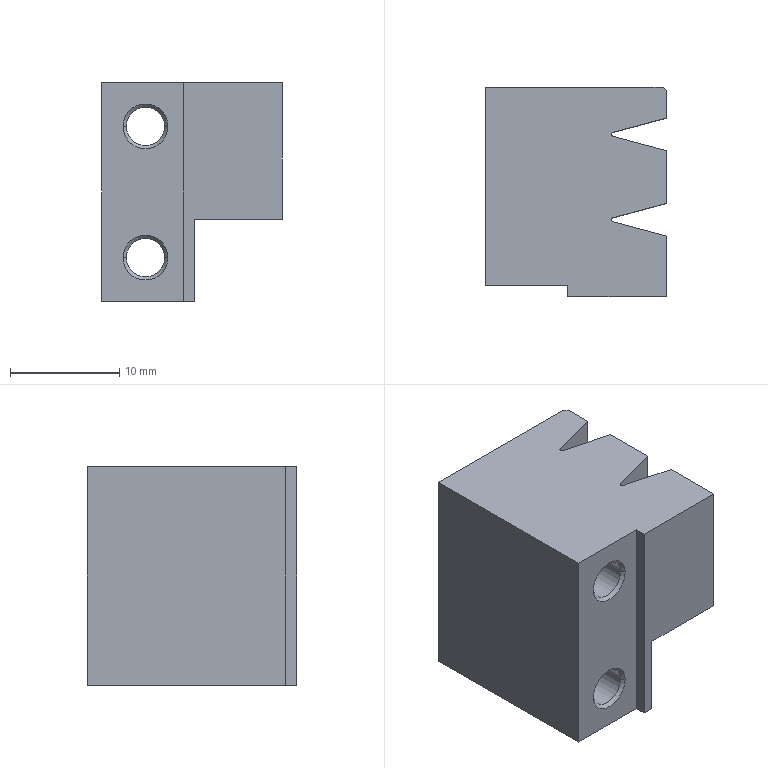Part | NX | 1 solid | 37 faces | box 16.5 x 19.1 x 20 mm | volume 4184 mm3 | plane 19 | cylinder 10 | cone 8 | commonest cylinder face diameters 3.5 x4 6 x4 0.4 x2
STEP:
#1=CARTESIAN_POINT('',(0.,9.05,-2.5));
#2=VERTEX_POINT('',#1);
#3=CARTESIAN_POINT('',(0.,-10.05,-2.5));
#4=VERTEX_POINT('',#3);
#5=CARTESIAN_POINT('',(0.,0.,-2.5));
#6=DIRECTION('',(0.,-1.,0.));
#7=VECTOR('',#6,1000.);
#8=LINE('',#5,#7);
#9=EDGE_CURVE('',#2,#4,#8,.T.);
#10=ORIENTED_EDGE('',*,*,#9,.F.);
#11=CARTESIAN_POINT('',(7.7,9.05,-2.5));
#12=VERTEX_POINT('',#11);
#13=CARTESIAN_POINT('',(0.,9.05,-2.5));
#14=DIRECTION('',(1.,0.,0.));
#15=VECTOR('',#14,1000.);
#16=LINE('',#13,#15);
#17=EDGE_CURVE('',#2,#12,#16,.T.);
#18=ORIENTED_EDGE('',*,*,#17,.T.);
#19=CARTESIAN_POINT('',(8.,8.75,-2.5));
#20=VERTEX_POINT('',#19);
#21=CARTESIAN_POINT('',(16.75,0.,-2.5));
#22=DIRECTION('',(-0.7071,0.7071,0.));
#23=VECTOR('',#22,1000.);
#24=LINE('',#21,#23);
#25=EDGE_CURVE('',#20,#12,#24,.T.);
#26=ORIENTED_EDGE('',*,*,#25,.F.);
#27=CARTESIAN_POINT('',(8.,6.247,-2.5));
#28=VERTEX_POINT('',#27);
#29=CARTESIAN_POINT('',(8.,0.,-2.5));
#30=DIRECTION('',(0.,1.,0.));
#31=VECTOR('',#30,1000.);
#32=LINE('',#29,#31);
#33=EDGE_CURVE('',#28,#20,#32,.T.);
#34=ORIENTED_EDGE('',*,*,#33,.F.);
#35=CARTESIAN_POINT('',(3.132,4.943,-2.5));
#36=VERTEX_POINT('',#35);
#37=CARTESIAN_POINT('',(0.,4.104,-2.5));
#38=DIRECTION('',(-0.9659,-0.2588,0.));
#39=VECTOR('',#38,1000.);
#40=LINE('',#37,#39);
#41=EDGE_CURVE('',#28,#36,#40,.T.);
#42=ORIENTED_EDGE('',*,*,#41,.T.);
#43=CARTESIAN_POINT('',(3.132,4.557,-2.5));
#44=VERTEX_POINT('',#43);
#45=CARTESIAN_POINT('',(3.184,4.75,-2.5));
#46=DIRECTION('',(0.,0.,-1.));
#47=DIRECTION('',(0.,1.,0.));
#48=AXIS2_PLACEMENT_3D('',#45,#46,#47);
#49=CIRCLE('',#48,0.2);
#50=EDGE_CURVE('',#44,#36,#49,.T.);
#51=ORIENTED_EDGE('',*,*,#50,.F.);
#52=CARTESIAN_POINT('',(8.,3.253,-2.5));
#53=VERTEX_POINT('',#52);
#54=CARTESIAN_POINT('',(0.,5.396,-2.5));
#55=DIRECTION('',(0.9659,-0.2588,0.));
#56=VECTOR('',#55,1000.);
#57=LINE('',#54,#56);
#58=EDGE_CURVE('',#44,#53,#57,.T.);
#59=ORIENTED_EDGE('',*,*,#58,.T.);
#60=CARTESIAN_POINT('',(8.,-1.553,-2.5));
#61=VERTEX_POINT('',#60);
#62=CARTESIAN_POINT('',(8.,0.,-2.5));
#63=DIRECTION('',(0.,1.,0.));
#64=VECTOR('',#63,1000.);
#65=LINE('',#62,#64);
#66=EDGE_CURVE('',#61,#53,#65,.T.);
#67=ORIENTED_EDGE('',*,*,#66,.F.);
#68=CARTESIAN_POINT('',(3.132,-2.857,-2.5));
#69=VERTEX_POINT('',#68);
#70=CARTESIAN_POINT('',(0.,-3.696,-2.5));
#71=DIRECTION('',(-0.9659,-0.2588,0.));
#72=VECTOR('',#71,1000.);
#73=LINE('',#70,#72);
#74=EDGE_CURVE('',#61,#69,#73,.T.);
#75=ORIENTED_EDGE('',*,*,#74,.T.);
#76=CARTESIAN_POINT('',(3.132,-3.243,-2.5));
#77=VERTEX_POINT('',#76);
#78=CARTESIAN_POINT('',(3.184,-3.05,-2.5));
#79=DIRECTION('',(0.,0.,-1.));
#80=DIRECTION('',(0.,1.,0.));
#81=AXIS2_PLACEMENT_3D('',#78,#79,#80);
#82=CIRCLE('',#81,0.2);
#83=EDGE_CURVE('',#77,#69,#82,.T.);
#84=ORIENTED_EDGE('',*,*,#83,.F.);
#85=CARTESIAN_POINT('',(8.,-4.547,-2.5));
#86=VERTEX_POINT('',#85);
#87=CARTESIAN_POINT('',(0.,-2.404,-2.5));
#88=DIRECTION('',(0.9659,-0.2588,0.));
#89=VECTOR('',#88,1000.);
#90=LINE('',#87,#89);
#91=EDGE_CURVE('',#77,#86,#90,.T.);
#92=ORIENTED_EDGE('',*,*,#91,.T.);
#93=CARTESIAN_POINT('',(8.,-10.05,-2.5));
#94=VERTEX_POINT('',#93);
#95=CARTESIAN_POINT('',(8.,0.,-2.5));
#96=DIRECTION('',(0.,1.,0.));
#97=VECTOR('',#96,1000.);
#98=LINE('',#95,#97);
#99=EDGE_CURVE('',#94,#86,#98,.T.);
#100=ORIENTED_EDGE('',*,*,#99,.F.);
#101=CARTESIAN_POINT('',(0.,-10.05,-2.5));
#102=DIRECTION('',(-1.,0.,0.));
#103=VECTOR('',#102,1000.);
#104=LINE('',#101,#103);
#105=EDGE_CURVE('',#94,#4,#104,.T.);
#106=ORIENTED_EDGE('',*,*,#105,.T.);
#107=EDGE_LOOP('',(#10,#18,#26,#34,#42,#51,#59,#67,#75,#84,#92,#100,#106));
#108=FACE_BOUND('',#107,.T.);
#109=CARTESIAN_POINT('',(8.7,-11.96,-2.5));
#110=DIRECTION('',(0.,0.,1.));
#111=DIRECTION('',(1.,0.,0.));
#112=AXIS2_PLACEMENT_3D('',#109,#110,#111);
#113=PLANE('',#112);
#114=ADVANCED_FACE('',(#108),#113,.F.);
#115=CARTESIAN_POINT('',(0.,-10.05,-10.));
#116=VERTEX_POINT('',#115);
#117=CARTESIAN_POINT('',(-1.,-10.05,-10.));
#118=VERTEX_POINT('',#117);
#119=CARTESIAN_POINT('',(0.,-10.05,-10.));
#120=DIRECTION('',(-1.,0.,0.));
#121=VECTOR('',#120,1000.);
#122=LINE('',#119,#121);
#123=EDGE_CURVE('',#116,#118,#122,.T.);
#124=ORIENTED_EDGE('',*,*,#123,.F.);
#125=CARTESIAN_POINT('',(0.,-10.05,0.));
#126=DIRECTION('',(0.,0.,-1.));
#127=VECTOR('',#126,1000.);
#128=LINE('',#125,#127);
#129=EDGE_CURVE('',#4,#116,#128,.T.);
#130=ORIENTED_EDGE('',*,*,#129,.F.);
#131=ORIENTED_EDGE('',*,*,#105,.F.);
#132=CARTESIAN_POINT('',(8.,-10.05,10.));
#133=VERTEX_POINT('',#132);
#134=CARTESIAN_POINT('',(8.,-10.05,0.));
#135=DIRECTION('',(0.,0.,1.));
#136=VECTOR('',#135,1000.);
#137=LINE('',#134,#136);
#138=EDGE_CURVE('',#94,#133,#137,.T.);
#139=ORIENTED_EDGE('',*,*,#138,.T.);
#140=CARTESIAN_POINT('',(-1.,-10.05,10.));
#141=VERTEX_POINT('',#140);
#142=CARTESIAN_POINT('',(0.,-10.05,10.));
#143=DIRECTION('',(-1.,0.,0.));
#144=VECTOR('',#143,1000.);
#145=LINE('',#142,#144);
#146=EDGE_CURVE('',#133,#141,#145,.T.);
#147=ORIENTED_EDGE('',*,*,#146,.T.);
#148=CARTESIAN_POINT('',(-1.,-10.05,0.));
#149=DIRECTION('',(0.,0.,1.));
#150=VECTOR('',#149,1000.);
#151=LINE('',#148,#150);
#152=EDGE_CURVE('',#118,#141,#151,.T.);
#153=ORIENTED_EDGE('',*,*,#152,.F.);
#154=EDGE_LOOP('',(#124,#130,#131,#139,#147,#153));
#155=FACE_BOUND('',#154,.T.);
#156=CARTESIAN_POINT('',(1.648,-10.05,2.608));
#157=DIRECTION('',(0.,-1.,0.));
#158=DIRECTION('',(0.,0.,-1.));
#159=AXIS2_PLACEMENT_3D('',#156,#157,#158);
#160=PLANE('',#159);
#161=ADVANCED_FACE('',(#155),#160,.T.);
#162=ORIENTED_EDGE('',*,*,#9,.T.);
#163=ORIENTED_EDGE('',*,*,#129,.T.);
#164=CARTESIAN_POINT('',(0.,9.05,-10.));
#165=VERTEX_POINT('',#164);
#166=CARTESIAN_POINT('',(0.,0.,-10.));
#167=DIRECTION('',(0.,-1.,0.));
#168=VECTOR('',#167,1000.);
#169=LINE('',#166,#168);
#170=EDGE_CURVE('',#165,#116,#169,.T.);
#171=ORIENTED_EDGE('',*,*,#170,.F.);
#172=CARTESIAN_POINT('',(0.,9.05,0.));
#173=DIRECTION('',(0.,0.,-1.));
#174=VECTOR('',#173,1000.);
#175=LINE('',#172,#174);
#176=EDGE_CURVE('',#2,#165,#175,.T.);
#177=ORIENTED_EDGE('',*,*,#176,.F.);
#178=EDGE_LOOP('',(#162,#163,#171,#177));
#179=FACE_BOUND('',#178,.T.);
#180=CARTESIAN_POINT('',(0.,-9.05,0.));
#181=DIRECTION('',(1.,0.,0.));
#182=DIRECTION('',(0.,1.,0.));
#183=AXIS2_PLACEMENT_3D('',#180,#181,#182);
#184=PLANE('',#183);
#185=ADVANCED_FACE('',(#179),#184,.T.);
#186=ORIENTED_EDGE('',*,*,#66,.T.);
#187=CARTESIAN_POINT('',(8.,3.253,10.));
#188=VERTEX_POINT('',#187);
#189=CARTESIAN_POINT('',(8.,3.253,0.));
#190=DIRECTION('',(0.,0.,-1.));
#191=VECTOR('',#190,1000.);
#192=LINE('',#189,#191);
#193=EDGE_CURVE('',#188,#53,#192,.T.);
#194=ORIENTED_EDGE('',*,*,#193,.F.);
#195=CARTESIAN_POINT('',(8.,-1.553,10.));
#196=VERTEX_POINT('',#195);
#197=CARTESIAN_POINT('',(8.,0.,10.));
#198=DIRECTION('',(0.,1.,0.));
#199=VECTOR('',#198,1000.);
#200=LINE('',#197,#199);
#201=EDGE_CURVE('',#196,#188,#200,.T.);
#202=ORIENTED_EDGE('',*,*,#201,.F.);
#203=CARTESIAN_POINT('',(8.,-1.553,0.));
#204=DIRECTION('',(0.,0.,-1.));
#205=VECTOR('',#204,1000.);
#206=LINE('',#203,#205);
#207=EDGE_CURVE('',#196,#61,#206,.T.);
#208=ORIENTED_EDGE('',*,*,#207,.T.);
#209=EDGE_LOOP('',(#186,#194,#202,#208));
#210=FACE_BOUND('',#209,.T.);
#211=CARTESIAN_POINT('',(8.,5.432,0.));
#212=DIRECTION('',(1.,0.,0.));
#213=DIRECTION('',(0.,1.,0.));
#214=AXIS2_PLACEMENT_3D('',#211,#212,#213);
#215=PLANE('',#214);
#216=ADVANCED_FACE('',(#210),#215,.T.);
#217=CARTESIAN_POINT('',(-1.,-9.05,10.));
#218=VERTEX_POINT('',#217);
#219=CARTESIAN_POINT('',(-1.,0.,10.));
#220=DIRECTION('',(0.,1.,0.));
#221=VECTOR('',#220,1000.);
#222=LINE('',#219,#221);
#223=EDGE_CURVE('',#141,#218,#222,.T.);
#224=ORIENTED_EDGE('',*,*,#223,.F.);
#225=ORIENTED_EDGE('',*,*,#146,.F.);
#226=CARTESIAN_POINT('',(8.,-4.547,10.));
#227=VERTEX_POINT('',#226);
#228=CARTESIAN_POINT('',(8.,0.,10.));
#229=DIRECTION('',(0.,-1.,0.));
#230=VECTOR('',#229,1000.);
#231=LINE('',#228,#230);
#232=EDGE_CURVE('',#227,#133,#231,.T.);
#233=ORIENTED_EDGE('',*,*,#232,.F.);
#234=CARTESIAN_POINT('',(3.132,-3.243,10.));
#235=VERTEX_POINT('',#234);
#236=CARTESIAN_POINT('',(0.,-2.404,10.));
#237=DIRECTION('',(-0.9659,0.2588,0.));
#238=VECTOR('',#237,1000.);
#239=LINE('',#236,#238);
#240=EDGE_CURVE('',#227,#235,#239,.T.);
#241=ORIENTED_EDGE('',*,*,#240,.T.);
#242=CARTESIAN_POINT('',(3.132,-2.857,10.));
#243=VERTEX_POINT('',#242);
#244=CARTESIAN_POINT('',(3.184,-3.05,10.));
#245=DIRECTION('',(0.,0.,-1.));
#246=DIRECTION('',(0.,1.,0.));
#247=AXIS2_PLACEMENT_3D('',#244,#245,#246);
#248=CIRCLE('',#247,0.2);
#249=EDGE_CURVE('',#235,#243,#248,.T.);
#250=ORIENTED_EDGE('',*,*,#249,.T.);
#251=CARTESIAN_POINT('',(0.,-3.696,10.));
#252=DIRECTION('',(0.9659,0.2588,0.));
#253=VECTOR('',#252,1000.);
#254=LINE('',#251,#253);
#255=EDGE_CURVE('',#243,#196,#254,.T.);
#256=ORIENTED_EDGE('',*,*,#255,.T.);
#257=ORIENTED_EDGE('',*,*,#201,.T.);
#258=CARTESIAN_POINT('',(3.132,4.557,10.));
#259=VERTEX_POINT('',#258);
#260=CARTESIAN_POINT('',(0.,5.396,10.));
#261=DIRECTION('',(0.9659,-0.2588,0.));
#262=VECTOR('',#261,1000.);
#263=LINE('',#260,#262);
#264=EDGE_CURVE('',#259,#188,#263,.T.);
#265=ORIENTED_EDGE('',*,*,#264,.F.);
#266=CARTESIAN_POINT('',(3.132,4.943,10.));
#267=VERTEX_POINT('',#266);
#268=CARTESIAN_POINT('',(3.184,4.75,10.));
#269=DIRECTION('',(0.,0.,-1.));
#270=DIRECTION('',(0.,1.,0.));
#271=AXIS2_PLACEMENT_3D('',#268,#269,#270);
#272=CIRCLE('',#271,0.2);
#273=EDGE_CURVE('',#259,#267,#272,.T.);
#274=ORIENTED_EDGE('',*,*,#273,.T.);
#275=CARTESIAN_POINT('',(8.,6.247,10.));
#276=VERTEX_POINT('',#275);
#277=CARTESIAN_POINT('',(0.,4.104,10.));
#278=DIRECTION('',(0.9659,0.2588,0.));
#279=VECTOR('',#278,1000.);
#280=LINE('',#277,#279);
#281=EDGE_CURVE('',#267,#276,#280,.T.);
#282=ORIENTED_EDGE('',*,*,#281,.T.);
#283=CARTESIAN_POINT('',(8.,8.75,10.));
#284=VERTEX_POINT('',#283);
#285=CARTESIAN_POINT('',(8.,0.,10.));
#286=DIRECTION('',(0.,1.,0.));
#287=VECTOR('',#286,1000.);
#288=LINE('',#285,#287);
#289=EDGE_CURVE('',#276,#284,#288,.T.);
#290=ORIENTED_EDGE('',*,*,#289,.T.);
#291=CARTESIAN_POINT('',(7.7,9.05,10.));
#292=VERTEX_POINT('',#291);
#293=CARTESIAN_POINT('',(16.75,0.,10.));
#294=DIRECTION('',(-0.7071,0.7071,0.));
#295=VECTOR('',#294,1000.);
#296=LINE('',#293,#295);
#297=EDGE_CURVE('',#284,#292,#296,.T.);
#298=ORIENTED_EDGE('',*,*,#297,.T.);
#299=CARTESIAN_POINT('',(-8.5,9.05,10.));
#300=VERTEX_POINT('',#299);
#301=CARTESIAN_POINT('',(0.,9.05,10.));
#302=DIRECTION('',(1.,0.,0.));
#303=VECTOR('',#302,1000.);
#304=LINE('',#301,#303);
#305=EDGE_CURVE('',#300,#292,#304,.T.);
#306=ORIENTED_EDGE('',*,*,#305,.F.);
#307=CARTESIAN_POINT('',(-8.5,-9.05,10.));
#308=VERTEX_POINT('',#307);
#309=CARTESIAN_POINT('',(-8.5,0.,10.));
#310=DIRECTION('',(0.,1.,0.));
#311=VECTOR('',#310,1000.);
#312=LINE('',#309,#311);
#313=EDGE_CURVE('',#308,#300,#312,.T.);
#314=ORIENTED_EDGE('',*,*,#313,.F.);
#315=CARTESIAN_POINT('',(0.,-9.05,10.));
#316=DIRECTION('',(-1.,0.,0.));
#317=VECTOR('',#316,1000.);
#318=LINE('',#315,#317);
#319=EDGE_CURVE('',#218,#308,#318,.T.);
#320=ORIENTED_EDGE('',*,*,#319,.F.);
#321=EDGE_LOOP('',(#224,#225,#233,#241,#250,#256,#257,#265,#274,#282,#290,#298,#306,#314,#320));
#322=FACE_BOUND('',#321,.T.);
#323=CARTESIAN_POINT('',(-1.,-9.05,10.));
#324=DIRECTION('',(0.,0.,1.));
#325=DIRECTION('',(1.,0.,0.));
#326=AXIS2_PLACEMENT_3D('',#323,#324,#325);
#327=PLANE('',#326);
#328=ADVANCED_FACE('',(#322),#327,.T.);
#329=CARTESIAN_POINT('',(-6.55,-9.05,-6.));
#330=VERTEX_POINT('',#329);
#331=CARTESIAN_POINT('',(-2.45,-9.05,-6.));
#332=VERTEX_POINT('',#331);
#333=CARTESIAN_POINT('',(-4.5,-9.05,-6.));
#334=DIRECTION('',(0.,-1.,0.));
#335=DIRECTION('',(-1.,0.,0.));
#336=AXIS2_PLACEMENT_3D('',#333,#334,#335);
#337=CIRCLE('',#336,2.05);
#338=EDGE_CURVE('',#330,#332,#337,.T.);
#339=ORIENTED_EDGE('',*,*,#338,.T.);
#340=CARTESIAN_POINT('',(-2.75,-8.75,-6.));
#341=VERTEX_POINT('',#340);
#342=CARTESIAN_POINT('',(-2.45,-9.05,-6.));
#343=DIRECTION('',(0.7071,-0.7071,0.));
#344=VECTOR('',#343,1000.);
#345=LINE('',#342,#344);
#346=EDGE_CURVE('',#332,#341,#345,.F.);
#347=ORIENTED_EDGE('',*,*,#346,.T.);
#348=CARTESIAN_POINT('',(-6.25,-8.75,-6.));
#349=VERTEX_POINT('',#348);
#350=CARTESIAN_POINT('',(-4.5,-8.75,-6.));
#351=DIRECTION('',(0.,-1.,0.));
#352=DIRECTION('',(-1.,0.,0.));
#353=AXIS2_PLACEMENT_3D('',#350,#351,#352);
#354=CIRCLE('',#353,1.75);
#355=EDGE_CURVE('',#349,#341,#354,.T.);
#356=ORIENTED_EDGE('',*,*,#355,.F.);
#357=CARTESIAN_POINT('',(-6.55,-9.05,-6.));
#358=DIRECTION('',(-0.7071,-0.7071,0.));
#359=VECTOR('',#358,1000.);
#360=LINE('',#357,#359);
#361=EDGE_CURVE('',#330,#349,#360,.F.);
#362=ORIENTED_EDGE('',*,*,#361,.F.);
#363=EDGE_LOOP('',(#339,#347,#356,#362));
#364=FACE_BOUND('',#363,.T.);
#365=CARTESIAN_POINT('',(-4.5,-9.05,-6.));
#366=DIRECTION('',(0.,-1.,0.));
#367=DIRECTION('',(-1.,0.,0.));
#368=AXIS2_PLACEMENT_3D('',#365,#366,#367);
#369=CONICAL_SURFACE('',#368,2.05,0.7854);
#370=ADVANCED_FACE('',(#364),#369,.F.);
#371=CARTESIAN_POINT('',(7.7,9.05,0.));
#372=DIRECTION('',(0.,0.,-1.));
#373=VECTOR('',#372,1000.);
#374=LINE('',#371,#373);
#375=EDGE_CURVE('',#292,#12,#374,.T.);
#376=ORIENTED_EDGE('',*,*,#375,.T.);
#377=ORIENTED_EDGE('',*,*,#17,.F.);
#378=ORIENTED_EDGE('',*,*,#176,.T.);
#379=CARTESIAN_POINT('',(-8.5,9.05,-10.));
#380=VERTEX_POINT('',#379);
#381=CARTESIAN_POINT('',(0.,9.05,-10.));
#382=DIRECTION('',(1.,0.,0.));
#383=VECTOR('',#382,1000.);
#384=LINE('',#381,#383);
#385=EDGE_CURVE('',#380,#165,#384,.T.);
#386=ORIENTED_EDGE('',*,*,#385,.F.);
#387=CARTESIAN_POINT('',(-8.5,9.05,0.));
#388=DIRECTION('',(0.,0.,-1.));
#389=VECTOR('',#388,1000.);
#390=LINE('',#387,#389);
#391=EDGE_CURVE('',#300,#380,#390,.T.);
#392=ORIENTED_EDGE('',*,*,#391,.F.);
#393=ORIENTED_EDGE('',*,*,#305,.T.);
#394=EDGE_LOOP('',(#376,#377,#378,#386,#392,#393));
#395=FACE_BOUND('',#394,.T.);
#396=CARTESIAN_POINT('',(-1.2,9.05,6.));
#397=VERTEX_POINT('',#396);
#398=CARTESIAN_POINT('',(-7.8,9.05,6.));
#399=VERTEX_POINT('',#398);
#400=CARTESIAN_POINT('',(-4.5,9.05,6.));
#401=DIRECTION('',(0.,1.,0.));
#402=DIRECTION('',(1.,0.,0.));
#403=AXIS2_PLACEMENT_3D('',#400,#401,#402);
#404=CIRCLE('',#403,3.3);
#405=EDGE_CURVE('',#397,#399,#404,.T.);
#406=ORIENTED_EDGE('',*,*,#405,.F.);
#407=CARTESIAN_POINT('',(-4.5,9.05,6.));
#408=DIRECTION('',(0.,1.,0.));
#409=DIRECTION('',(1.,0.,0.));
#410=AXIS2_PLACEMENT_3D('',#407,#408,#409);
#411=CIRCLE('',#410,3.3);
#412=EDGE_CURVE('',#399,#397,#411,.T.);
#413=ORIENTED_EDGE('',*,*,#412,.F.);
#414=EDGE_LOOP('',(#406,#413));
#415=FACE_BOUND('',#414,.T.);
#416=CARTESIAN_POINT('',(-7.8,9.05,-6.));
#417=VERTEX_POINT('',#416);
#418=CARTESIAN_POINT('',(-1.2,9.05,-6.));
#419=VERTEX_POINT('',#418);
#420=CARTESIAN_POINT('',(-4.5,9.05,-6.));
#421=DIRECTION('',(0.,1.,0.));
#422=DIRECTION('',(1.,0.,0.));
#423=AXIS2_PLACEMENT_3D('',#420,#421,#422);
#424=CIRCLE('',#423,3.3);
#425=EDGE_CURVE('',#417,#419,#424,.T.);
#426=ORIENTED_EDGE('',*,*,#425,.F.);
#427=CARTESIAN_POINT('',(-4.5,9.05,-6.));
#428=DIRECTION('',(0.,1.,0.));
#429=DIRECTION('',(1.,0.,0.));
#430=AXIS2_PLACEMENT_3D('',#427,#428,#429);
#431=CIRCLE('',#430,3.3);
#432=EDGE_CURVE('',#419,#417,#431,.T.);
#433=ORIENTED_EDGE('',*,*,#432,.F.);
#434=EDGE_LOOP('',(#426,#433));
#435=FACE_BOUND('',#434,.T.);
#436=CARTESIAN_POINT('',(8.,9.05,-10.));
#437=DIRECTION('',(0.,1.,0.));
#438=DIRECTION('',(1.,0.,0.));
#439=AXIS2_PLACEMENT_3D('',#436,#437,#438);
#440=PLANE('',#439);
#441=ADVANCED_FACE('',(#395,#415,#435),#440,.T.);
#442=CARTESIAN_POINT('',(-4.5,1.95,-3.));
#443=VERTEX_POINT('',#442);
#444=CARTESIAN_POINT('',(-4.5,1.95,-9.));
#445=VERTEX_POINT('',#444);
#446=CARTESIAN_POINT('',(-4.5,1.95,-6.));
#447=DIRECTION('',(0.,1.,0.));
#448=DIRECTION('',(0.,0.,1.));
#449=AXIS2_PLACEMENT_3D('',#446,#447,#448);
#450=CIRCLE('',#449,3.);
#451=EDGE_CURVE('',#443,#445,#450,.T.);
#452=ORIENTED_EDGE('',*,*,#451,.T.);
#453=CARTESIAN_POINT('',(-4.5,1.95,-6.));
#454=DIRECTION('',(0.,1.,0.));
#455=DIRECTION('',(0.,0.,1.));
#456=AXIS2_PLACEMENT_3D('',#453,#454,#455);
#457=CIRCLE('',#456,3.);
#458=EDGE_CURVE('',#445,#443,#457,.T.);
#459=ORIENTED_EDGE('',*,*,#458,.T.);
#460=EDGE_LOOP('',(#452,#459));
#461=FACE_BOUND('',#460,.T.);
#462=CARTESIAN_POINT('',(-2.75,1.95,-6.));
#463=VERTEX_POINT('',#462);
#464=CARTESIAN_POINT('',(-6.25,1.95,-6.));
#465=VERTEX_POINT('',#464);
#466=CARTESIAN_POINT('',(-4.5,1.95,-6.));
#467=DIRECTION('',(0.,1.,0.));
#468=DIRECTION('',(-1.,0.,0.));
#469=AXIS2_PLACEMENT_3D('',#466,#467,#468);
#470=CIRCLE('',#469,1.75);
#471=EDGE_CURVE('',#463,#465,#470,.T.);
#472=ORIENTED_EDGE('',*,*,#471,.F.);
#473=CARTESIAN_POINT('',(-4.5,1.95,-6.));
#474=DIRECTION('',(0.,1.,0.));
#475=DIRECTION('',(-1.,0.,0.));
#476=AXIS2_PLACEMENT_3D('',#473,#474,#475);
#477=CIRCLE('',#476,1.75);
#478=EDGE_CURVE('',#465,#463,#477,.T.);
#479=ORIENTED_EDGE('',*,*,#478,.F.);
#480=EDGE_LOOP('',(#472,#479));
#481=FACE_BOUND('',#480,.T.);
#482=CARTESIAN_POINT('',(-1.269,1.95,6.939));
#483=DIRECTION('',(0.,1.,0.));
#484=DIRECTION('',(1.,0.,0.));
#485=AXIS2_PLACEMENT_3D('',#482,#483,#484);
#486=PLANE('',#485);
#487=ADVANCED_FACE('',(#461,#481),#486,.T.);
#488=CARTESIAN_POINT('',(-1.5,8.75,6.));
#489=VERTEX_POINT('',#488);
#490=CARTESIAN_POINT('',(-4.5,8.75,3.));
#491=VERTEX_POINT('',#490);
#492=CARTESIAN_POINT('',(-4.5,8.75,6.));
#493=DIRECTION('',(0.,1.,0.));
#494=DIRECTION('',(1.,0.,0.));
#495=AXIS2_PLACEMENT_3D('',#492,#493,#494);
#496=CIRCLE('',#495,3.);
#497=EDGE_CURVE('',#489,#491,#496,.T.);
#498=ORIENTED_EDGE('',*,*,#497,.F.);
#499=CARTESIAN_POINT('',(-1.5,8.75,6.));
#500=DIRECTION('',(0.7071,0.7071,0.));
#501=VECTOR('',#500,1000.);
#502=LINE('',#499,#501);
#503=EDGE_CURVE('',#397,#489,#502,.F.);
#504=ORIENTED_EDGE('',*,*,#503,.F.);
#505=ORIENTED_EDGE('',*,*,#405,.T.);
#506=CARTESIAN_POINT('',(-7.5,8.75,6.));
#507=VERTEX_POINT('',#506);
#508=CARTESIAN_POINT('',(-7.5,8.75,6.));
#509=DIRECTION('',(-0.7071,0.7071,0.));
#510=VECTOR('',#509,1000.);
#511=LINE('',#508,#510);
#512=EDGE_CURVE('',#399,#507,#511,.F.);
#513=ORIENTED_EDGE('',*,*,#512,.T.);
#514=CARTESIAN_POINT('',(-4.5,8.75,6.));
#515=DIRECTION('',(0.,1.,0.));
#516=DIRECTION('',(1.,0.,0.));
#517=AXIS2_PLACEMENT_3D('',#514,#515,#516);
#518=CIRCLE('',#517,3.);
#519=EDGE_CURVE('',#491,#507,#518,.T.);
#520=ORIENTED_EDGE('',*,*,#519,.F.);
#521=EDGE_LOOP('',(#498,#504,#505,#513,#520));
#522=FACE_BOUND('',#521,.T.);
#523=CARTESIAN_POINT('',(-4.5,8.75,6.));
#524=DIRECTION('',(0.,1.,0.));
#525=DIRECTION('',(1.,0.,0.));
#526=AXIS2_PLACEMENT_3D('',#523,#524,#525);
#527=CONICAL_SURFACE('',#526,3.,0.7854);
#528=ADVANCED_FACE('',(#522),#527,.F.);
#529=CARTESIAN_POINT('',(-6.55,-9.05,6.));
#530=VERTEX_POINT('',#529);
#531=CARTESIAN_POINT('',(-2.45,-9.05,6.));
#532=VERTEX_POINT('',#531);
#533=CARTESIAN_POINT('',(-4.5,-9.05,6.));
#534=DIRECTION('',(0.,-1.,0.));
#535=DIRECTION('',(-1.,0.,0.));
#536=AXIS2_PLACEMENT_3D('',#533,#534,#535);
#537=CIRCLE('',#536,2.05);
#538=EDGE_CURVE('',#530,#532,#537,.T.);
#539=ORIENTED_EDGE('',*,*,#538,.T.);
#540=CARTESIAN_POINT('',(-2.75,-8.75,6.));
#541=VERTEX_POINT('',#540);
#542=CARTESIAN_POINT('',(-2.45,-9.05,6.));
#543=DIRECTION('',(0.7071,-0.7071,0.));
#544=VECTOR('',#543,1000.);
#545=LINE('',#542,#544);
#546=EDGE_CURVE('',#532,#541,#545,.F.);
#547=ORIENTED_EDGE('',*,*,#546,.T.);
#548=CARTESIAN_POINT('',(-6.25,-8.75,6.));
#549=VERTEX_POINT('',#548);
#550=CARTESIAN_POINT('',(-4.5,-8.75,6.));
#551=DIRECTION('',(0.,-1.,0.));
#552=DIRECTION('',(-1.,0.,0.));
#553=AXIS2_PLACEMENT_3D('',#550,#551,#552);
#554=CIRCLE('',#553,1.75);
#555=EDGE_CURVE('',#549,#541,#554,.T.);
#556=ORIENTED_EDGE('',*,*,#555,.F.);
#557=CARTESIAN_POINT('',(-6.55,-9.05,6.));
#558=DIRECTION('',(-0.7071,-0.7071,0.));
#559=VECTOR('',#558,1000.);
#560=LINE('',#557,#559);
#561=EDGE_CURVE('',#530,#549,#560,.F.);
#562=ORIENTED_EDGE('',*,*,#561,.F.);
#563=EDGE_LOOP('',(#539,#547,#556,#562));
#564=FACE_BOUND('',#563,.T.);
#565=CARTESIAN_POINT('',(-4.5,-9.05,6.));
#566=DIRECTION('',(0.,-1.,0.));
#567=DIRECTION('',(-1.,0.,0.));
#568=AXIS2_PLACEMENT_3D('',#565,#566,#567);
#569=CONICAL_SURFACE('',#568,2.05,0.7854);
#570=ADVANCED_FACE('',(#564),#569,.F.);
#571=ORIENTED_EDGE('',*,*,#313,.T.);
#572=ORIENTED_EDGE('',*,*,#391,.T.);
#573=CARTESIAN_POINT('',(-8.5,-9.05,-10.));
#574=VERTEX_POINT('',#573);
#575=CARTESIAN_POINT('',(-8.5,0.,-10.));
#576=DIRECTION('',(0.,1.,0.));
#577=VECTOR('',#576,1000.);
#578=LINE('',#575,#577);
#579=EDGE_CURVE('',#574,#380,#578,.T.);
#580=ORIENTED_EDGE('',*,*,#579,.F.);
#581=CARTESIAN_POINT('',(-8.5,-9.05,0.));
#582=DIRECTION('',(0.,0.,1.));
#583=VECTOR('',#582,1000.);
#584=LINE('',#581,#583);
#585=EDGE_CURVE('',#574,#308,#584,.T.);
#586=ORIENTED_EDGE('',*,*,#585,.T.);
#587=EDGE_LOOP('',(#571,#572,#580,#586));
#588=FACE_BOUND('',#587,.T.);
#589=CARTESIAN_POINT('',(-8.5,9.05,-10.));
#590=DIRECTION('',(-1.,0.,0.));
#591=DIRECTION('',(0.,0.,1.));
#592=AXIS2_PLACEMENT_3D('',#589,#590,#591);
#593=PLANE('',#592);
#594=ADVANCED_FACE('',(#588),#593,.T.);
#595=CARTESIAN_POINT('',(-1.,-9.05,-10.));
#596=VERTEX_POINT('',#595);
#597=CARTESIAN_POINT('',(-1.,-9.05,0.));
#598=DIRECTION('',(0.,0.,-1.));
#599=VECTOR('',#598,1000.);
#600=LINE('',#597,#599);
#601=EDGE_CURVE('',#218,#596,#600,.T.);
#602=ORIENTED_EDGE('',*,*,#601,.F.);
#603=ORIENTED_EDGE('',*,*,#319,.T.);
#604=ORIENTED_EDGE('',*,*,#585,.F.);
#605=CARTESIAN_POINT('',(0.,-9.05,-10.));
#606=DIRECTION('',(1.,0.,0.));
#607=VECTOR('',#606,1000.);
#608=LINE('',#605,#607);
#609=EDGE_CURVE('',#574,#596,#608,.T.);
#610=ORIENTED_EDGE('',*,*,#609,.T.);
#611=EDGE_LOOP('',(#602,#603,#604,#610));
#612=FACE_BOUND('',#611,.T.);
#613=ORIENTED_EDGE('',*,*,#538,.F.);
#614=CARTESIAN_POINT('',(-4.5,-9.05,6.));
#615=DIRECTION('',(0.,-1.,0.));
#616=DIRECTION('',(-1.,0.,0.));
#617=AXIS2_PLACEMENT_3D('',#614,#615,#616);
#618=CIRCLE('',#617,2.05);
#619=EDGE_CURVE('',#532,#530,#618,.T.);
#620=ORIENTED_EDGE('',*,*,#619,.F.);
#621=EDGE_LOOP('',(#613,#620));
#622=FACE_BOUND('',#621,.T.);
#623=ORIENTED_EDGE('',*,*,#338,.F.);
#624=CARTESIAN_POINT('',(-4.5,-9.05,-6.));
#625=DIRECTION('',(0.,-1.,0.));
#626=DIRECTION('',(-1.,0.,0.));
#627=AXIS2_PLACEMENT_3D('',#624,#625,#626);
#628=CIRCLE('',#627,2.05);
#629=EDGE_CURVE('',#332,#330,#628,.T.);
#630=ORIENTED_EDGE('',*,*,#629,.F.);
#631=EDGE_LOOP('',(#623,#630));
#632=FACE_BOUND('',#631,.T.);
#633=CARTESIAN_POINT('',(-8.,-9.05,-10.));
#634=DIRECTION('',(0.,-1.,0.));
#635=DIRECTION('',(0.,0.,-1.));
#636=AXIS2_PLACEMENT_3D('',#633,#634,#635);
#637=PLANE('',#636);
#638=ADVANCED_FACE('',(#612,#622,#632),#637,.T.);
#639=ORIENTED_EDGE('',*,*,#451,.F.);
#640=CARTESIAN_POINT('',(-4.5,8.75,-3.));
#641=VERTEX_POINT('',#640);
#642=CARTESIAN_POINT('',(-4.5,9.05,-3.));
#643=DIRECTION('',(0.,1.,0.));
#644=VECTOR('',#643,1000.);
#645=LINE('',#642,#644);
#646=EDGE_CURVE('',#443,#641,#645,.T.);
#647=ORIENTED_EDGE('',*,*,#646,.T.);
#648=CARTESIAN_POINT('',(-1.5,8.75,-6.));
#649=VERTEX_POINT('',#648);
#650=CARTESIAN_POINT('',(-4.5,8.75,-6.));
#651=DIRECTION('',(0.,1.,0.));
#652=DIRECTION('',(1.,0.,0.));
#653=AXIS2_PLACEMENT_3D('',#650,#651,#652);
#654=CIRCLE('',#653,3.);
#655=EDGE_CURVE('',#641,#649,#654,.T.);
#656=ORIENTED_EDGE('',*,*,#655,.T.);
#657=CARTESIAN_POINT('',(-4.5,8.75,-9.));
#658=VERTEX_POINT('',#657);
#659=CARTESIAN_POINT('',(-4.5,8.75,-6.));
#660=DIRECTION('',(0.,1.,0.));
#661=DIRECTION('',(1.,0.,0.));
#662=AXIS2_PLACEMENT_3D('',#659,#660,#661);
#663=CIRCLE('',#662,3.);
#664=EDGE_CURVE('',#649,#658,#663,.T.);
#665=ORIENTED_EDGE('',*,*,#664,.T.);
#666=CARTESIAN_POINT('',(-4.5,9.05,-9.));
#667=DIRECTION('',(0.,1.,0.));
#668=VECTOR('',#667,1000.);
#669=LINE('',#666,#668);
#670=EDGE_CURVE('',#445,#658,#669,.T.);
#671=ORIENTED_EDGE('',*,*,#670,.F.);
#672=EDGE_LOOP('',(#639,#647,#656,#665,#671));
#673=FACE_BOUND('',#672,.T.);
#674=CARTESIAN_POINT('',(-4.5,9.05,-6.));
#675=DIRECTION('',(0.,1.,0.));
#676=DIRECTION('',(0.,0.,1.));
#677=AXIS2_PLACEMENT_3D('',#674,#675,#676);
#678=CYLINDRICAL_SURFACE('',#677,3.);
#679=ADVANCED_FACE('',(#673),#678,.F.);
#680=CARTESIAN_POINT('',(-6.25,1.95,6.));
#681=VERTEX_POINT('',#680);
#682=CARTESIAN_POINT('',(-2.75,1.95,6.));
#683=VERTEX_POINT('',#682);
#684=CARTESIAN_POINT('',(-4.5,1.95,6.));
#685=DIRECTION('',(0.,1.,0.));
#686=DIRECTION('',(-1.,0.,0.));
#687=AXIS2_PLACEMENT_3D('',#684,#685,#686);
#688=CIRCLE('',#687,1.75);
#689=EDGE_CURVE('',#681,#683,#688,.T.);
#690=ORIENTED_EDGE('',*,*,#689,.T.);
#691=CARTESIAN_POINT('',(-2.75,-9.05,6.));
#692=DIRECTION('',(0.,1.,0.));
#693=VECTOR('',#692,1000.);
#694=LINE('',#691,#693);
#695=EDGE_CURVE('',#541,#683,#694,.T.);
#696=ORIENTED_EDGE('',*,*,#695,.F.);
#697=CARTESIAN_POINT('',(-4.5,-8.75,6.));
#698=DIRECTION('',(0.,-1.,0.));
#699=DIRECTION('',(-1.,0.,0.));
#700=AXIS2_PLACEMENT_3D('',#697,#698,#699);
#701=CIRCLE('',#700,1.75);
#702=EDGE_CURVE('',#541,#549,#701,.T.);
#703=ORIENTED_EDGE('',*,*,#702,.T.);
#704=CARTESIAN_POINT('',(-6.25,-9.05,6.));
#705=DIRECTION('',(0.,1.,0.));
#706=VECTOR('',#705,1000.);
#707=LINE('',#704,#706);
#708=EDGE_CURVE('',#549,#681,#707,.T.);
#709=ORIENTED_EDGE('',*,*,#708,.T.);
#710=EDGE_LOOP('',(#690,#696,#703,#709));
#711=FACE_BOUND('',#710,.T.);
#712=CARTESIAN_POINT('',(-4.5,-9.05,6.));
#713=DIRECTION('',(0.,1.,0.));
#714=DIRECTION('',(-1.,0.,0.));
#715=AXIS2_PLACEMENT_3D('',#712,#713,#714);
#716=CYLINDRICAL_SURFACE('',#715,1.75);
#717=ADVANCED_FACE('',(#711),#716,.F.);
#718=ORIENTED_EDGE('',*,*,#471,.T.);
#719=CARTESIAN_POINT('',(-6.25,-9.05,-6.));
#720=DIRECTION('',(0.,1.,0.));
#721=VECTOR('',#720,1000.);
#722=LINE('',#719,#721);
#723=EDGE_CURVE('',#465,#349,#722,.F.);
#724=ORIENTED_EDGE('',*,*,#723,.T.);
#725=ORIENTED_EDGE('',*,*,#355,.T.);
#726=CARTESIAN_POINT('',(-2.75,-9.05,-6.));
#727=DIRECTION('',(0.,1.,0.));
#728=VECTOR('',#727,1000.);
#729=LINE('',#726,#728);
#730=EDGE_CURVE('',#463,#341,#729,.F.);
#731=ORIENTED_EDGE('',*,*,#730,.F.);
#732=EDGE_LOOP('',(#718,#724,#725,#731));
#733=FACE_BOUND('',#732,.T.);
#734=CARTESIAN_POINT('',(-4.5,-9.05,-6.));
#735=DIRECTION('',(0.,1.,0.));
#736=DIRECTION('',(-1.,0.,0.));
#737=AXIS2_PLACEMENT_3D('',#734,#735,#736);
#738=CYLINDRICAL_SURFACE('',#737,1.75);
#739=ADVANCED_FACE('',(#733),#738,.F.);
#740=CARTESIAN_POINT('',(-4.5,1.95,9.));
#741=VERTEX_POINT('',#740);
#742=CARTESIAN_POINT('',(-4.5,1.95,3.));
#743=VERTEX_POINT('',#742);
#744=CARTESIAN_POINT('',(-4.5,1.95,6.));
#745=DIRECTION('',(0.,1.,0.));
#746=DIRECTION('',(0.,0.,1.));
#747=AXIS2_PLACEMENT_3D('',#744,#745,#746);
#748=CIRCLE('',#747,3.);
#749=EDGE_CURVE('',#741,#743,#748,.T.);
#750=ORIENTED_EDGE('',*,*,#749,.T.);
#751=CARTESIAN_POINT('',(-4.5,1.95,6.));
#752=DIRECTION('',(0.,1.,0.));
#753=DIRECTION('',(0.,0.,1.));
#754=AXIS2_PLACEMENT_3D('',#751,#752,#753);
#755=CIRCLE('',#754,3.);
#756=EDGE_CURVE('',#743,#741,#755,.T.);
#757=ORIENTED_EDGE('',*,*,#756,.T.);
#758=EDGE_LOOP('',(#750,#757));
#759=FACE_BOUND('',#758,.T.);
#760=ORIENTED_EDGE('',*,*,#689,.F.);
#761=CARTESIAN_POINT('',(-4.5,1.95,6.));
#762=DIRECTION('',(0.,1.,0.));
#763=DIRECTION('',(-1.,0.,0.));
#764=AXIS2_PLACEMENT_3D('',#761,#762,#763);
#765=CIRCLE('',#764,1.75);
#766=EDGE_CURVE('',#683,#681,#765,.T.);
#767=ORIENTED_EDGE('',*,*,#766,.F.);
#768=EDGE_LOOP('',(#760,#767));
#769=FACE_BOUND('',#768,.T.);
#770=CARTESIAN_POINT('',(-1.269,1.95,6.939));
#771=DIRECTION('',(0.,1.,0.));
#772=DIRECTION('',(1.,0.,0.));
#773=AXIS2_PLACEMENT_3D('',#770,#771,#772);
#774=PLANE('',#773);
#775=ADVANCED_FACE('',(#759,#769),#774,.T.);
#776=ORIENTED_EDGE('',*,*,#749,.F.);
#777=CARTESIAN_POINT('',(-4.5,8.75,9.));
#778=VERTEX_POINT('',#777);
#779=CARTESIAN_POINT('',(-4.5,9.05,9.));
#780=DIRECTION('',(0.,1.,0.));
#781=VECTOR('',#780,1000.);
#782=LINE('',#779,#781);
#783=EDGE_CURVE('',#741,#778,#782,.T.);
#784=ORIENTED_EDGE('',*,*,#783,.T.);
#785=CARTESIAN_POINT('',(-4.5,8.75,6.));
#786=DIRECTION('',(0.,1.,0.));
#787=DIRECTION('',(1.,0.,0.));
#788=AXIS2_PLACEMENT_3D('',#785,#786,#787);
#789=CIRCLE('',#788,3.);
#790=EDGE_CURVE('',#778,#489,#789,.T.);
#791=ORIENTED_EDGE('',*,*,#790,.T.);
#792=ORIENTED_EDGE('',*,*,#497,.T.);
#793=CARTESIAN_POINT('',(-4.5,9.05,3.));
#794=DIRECTION('',(0.,1.,0.));
#795=VECTOR('',#794,1000.);
#796=LINE('',#793,#795);
#797=EDGE_CURVE('',#743,#491,#796,.T.);
#798=ORIENTED_EDGE('',*,*,#797,.F.);
#799=EDGE_LOOP('',(#776,#784,#791,#792,#798));
#800=FACE_BOUND('',#799,.T.);
#801=CARTESIAN_POINT('',(-4.5,9.05,6.));
#802=DIRECTION('',(0.,1.,0.));
#803=DIRECTION('',(0.,0.,1.));
#804=AXIS2_PLACEMENT_3D('',#801,#802,#803);
#805=CYLINDRICAL_SURFACE('',#804,3.);
#806=ADVANCED_FACE('',(#800),#805,.F.);
#807=CARTESIAN_POINT('',(8.,6.247,0.));
#808=DIRECTION('',(0.,0.,-1.));
#809=VECTOR('',#808,1000.);
#810=LINE('',#807,#809);
#811=EDGE_CURVE('',#276,#28,#810,.T.);
#812=ORIENTED_EDGE('',*,*,#811,.T.);
#813=ORIENTED_EDGE('',*,*,#33,.T.);
#814=CARTESIAN_POINT('',(8.,8.75,0.));
#815=DIRECTION('',(0.,0.,1.));
#816=VECTOR('',#815,1000.);
#817=LINE('',#814,#816);
#818=EDGE_CURVE('',#20,#284,#817,.T.);
#819=ORIENTED_EDGE('',*,*,#818,.T.);
#820=ORIENTED_EDGE('',*,*,#289,.F.);
#821=EDGE_LOOP('',(#812,#813,#819,#820));
#822=FACE_BOUND('',#821,.T.);
#823=CARTESIAN_POINT('',(8.,5.532,0.));
#824=DIRECTION('',(1.,0.,0.));
#825=DIRECTION('',(0.,1.,0.));
#826=AXIS2_PLACEMENT_3D('',#823,#824,#825);
#827=PLANE('',#826);
#828=ADVANCED_FACE('',(#822),#827,.T.);
#829=ORIENTED_EDGE('',*,*,#273,.F.);
#830=CARTESIAN_POINT('',(3.132,4.557,12.));
#831=DIRECTION('',(0.,0.,-1.));
#832=VECTOR('',#831,1000.);
#833=LINE('',#830,#832);
#834=EDGE_CURVE('',#259,#44,#833,.T.);
#835=ORIENTED_EDGE('',*,*,#834,.T.);
#836=ORIENTED_EDGE('',*,*,#50,.T.);
#837=CARTESIAN_POINT('',(3.132,4.943,12.));
#838=DIRECTION('',(0.,0.,-1.));
#839=VECTOR('',#838,1000.);
#840=LINE('',#837,#839);
#841=EDGE_CURVE('',#267,#36,#840,.T.);
#842=ORIENTED_EDGE('',*,*,#841,.F.);
#843=EDGE_LOOP('',(#829,#835,#836,#842));
#844=FACE_BOUND('',#843,.T.);
#845=CARTESIAN_POINT('',(3.184,4.75,12.));
#846=DIRECTION('',(0.,0.,-1.));
#847=DIRECTION('',(0.,1.,0.));
#848=AXIS2_PLACEMENT_3D('',#845,#846,#847);
#849=CYLINDRICAL_SURFACE('',#848,0.2);
#850=ADVANCED_FACE('',(#844),#849,.F.);
#851=ORIENTED_EDGE('',*,*,#281,.F.);
#852=ORIENTED_EDGE('',*,*,#841,.T.);
#853=ORIENTED_EDGE('',*,*,#41,.F.);
#854=ORIENTED_EDGE('',*,*,#811,.F.);
#855=EDGE_LOOP('',(#851,#852,#853,#854));
#856=FACE_BOUND('',#855,.T.);
#857=CARTESIAN_POINT('',(8.868,6.48,12.));
#858=DIRECTION('',(-0.2588,0.9659,0.));
#859=DIRECTION('',(0.,0.,1.));
#860=AXIS2_PLACEMENT_3D('',#857,#858,#859);
#861=PLANE('',#860);
#862=ADVANCED_FACE('',(#856),#861,.F.);
#863=ORIENTED_EDGE('',*,*,#264,.T.);
#864=ORIENTED_EDGE('',*,*,#193,.T.);
#865=ORIENTED_EDGE('',*,*,#58,.F.);
#866=ORIENTED_EDGE('',*,*,#834,.F.);
#867=EDGE_LOOP('',(#863,#864,#865,#866));
#868=FACE_BOUND('',#867,.T.);
#869=CARTESIAN_POINT('',(3.132,4.557,12.));
#870=DIRECTION('',(-0.2588,-0.9659,0.));
#871=DIRECTION('',(-0.9659,0.2588,0.));
#872=AXIS2_PLACEMENT_3D('',#869,#870,#871);
#873=PLANE('',#872);
#874=ADVANCED_FACE('',(#868),#873,.F.);
#875=ORIENTED_EDGE('',*,*,#170,.T.);
#876=ORIENTED_EDGE('',*,*,#123,.T.);
#877=CARTESIAN_POINT('',(-1.,-9.05,-10.));
#878=DIRECTION('',(0.,-1.,0.));
#879=VECTOR('',#878,1000.);
#880=LINE('',#877,#879);
#881=EDGE_CURVE('',#596,#118,#880,.T.);
#882=ORIENTED_EDGE('',*,*,#881,.F.);
#883=ORIENTED_EDGE('',*,*,#609,.F.);
#884=ORIENTED_EDGE('',*,*,#579,.T.);
#885=ORIENTED_EDGE('',*,*,#385,.T.);
#886=EDGE_LOOP('',(#875,#876,#882,#883,#884,#885));
#887=FACE_BOUND('',#886,.T.);
#888=CARTESIAN_POINT('',(0.,-9.05,-10.));
#889=DIRECTION('',(0.,0.,-1.));
#890=DIRECTION('',(0.,-1.,0.));
#891=AXIS2_PLACEMENT_3D('',#888,#889,#890);
#892=PLANE('',#891);
#893=ADVANCED_FACE('',(#887),#892,.T.);
#894=ORIENTED_EDGE('',*,*,#425,.T.);
#895=CARTESIAN_POINT('',(-1.5,8.75,-6.));
#896=DIRECTION('',(0.7071,0.7071,0.));
#897=VECTOR('',#896,1000.);
#898=LINE('',#895,#897);
#899=EDGE_CURVE('',#419,#649,#898,.F.);
#900=ORIENTED_EDGE('',*,*,#899,.T.);
#901=ORIENTED_EDGE('',*,*,#655,.F.);
#902=CARTESIAN_POINT('',(-7.5,8.75,-6.));
#903=VERTEX_POINT('',#902);
#904=CARTESIAN_POINT('',(-4.5,8.75,-6.));
#905=DIRECTION('',(0.,1.,0.));
#906=DIRECTION('',(1.,0.,0.));
#907=AXIS2_PLACEMENT_3D('',#904,#905,#906);
#908=CIRCLE('',#907,3.);
#909=EDGE_CURVE('',#903,#641,#908,.T.);
#910=ORIENTED_EDGE('',*,*,#909,.F.);
#911=CARTESIAN_POINT('',(-7.5,8.75,-6.));
#912=DIRECTION('',(-0.7071,0.7071,0.));
#913=VECTOR('',#912,1000.);
#914=LINE('',#911,#913);
#915=EDGE_CURVE('',#417,#903,#914,.F.);
#916=ORIENTED_EDGE('',*,*,#915,.F.);
#917=EDGE_LOOP('',(#894,#900,#901,#910,#916));
#918=FACE_BOUND('',#917,.T.);
#919=CARTESIAN_POINT('',(-4.5,8.75,-6.));
#920=DIRECTION('',(0.,1.,0.));
#921=DIRECTION('',(1.,0.,0.));
#922=AXIS2_PLACEMENT_3D('',#919,#920,#921);
#923=CONICAL_SURFACE('',#922,3.,0.7854);
#924=ADVANCED_FACE('',(#918),#923,.F.);
#925=ORIENTED_EDGE('',*,*,#601,.T.);
#926=ORIENTED_EDGE('',*,*,#881,.T.);
#927=ORIENTED_EDGE('',*,*,#152,.T.);
#928=ORIENTED_EDGE('',*,*,#223,.T.);
#929=EDGE_LOOP('',(#925,#926,#927,#928));
#930=FACE_BOUND('',#929,.T.);
#931=CARTESIAN_POINT('',(-1.,-9.05,-10.));
#932=DIRECTION('',(-1.,0.,0.));
#933=DIRECTION('',(0.,0.,1.));
#934=AXIS2_PLACEMENT_3D('',#931,#932,#933);
#935=PLANE('',#934);
#936=ADVANCED_FACE('',(#930),#935,.T.);
#937=ORIENTED_EDGE('',*,*,#375,.F.);
#938=ORIENTED_EDGE('',*,*,#297,.F.);
#939=ORIENTED_EDGE('',*,*,#818,.F.);
#940=ORIENTED_EDGE('',*,*,#25,.T.);
#941=EDGE_LOOP('',(#937,#938,#939,#940));
#942=FACE_BOUND('',#941,.T.);
#943=CARTESIAN_POINT('',(7.85,8.9,3.75));
#944=DIRECTION('',(-0.7071,-0.7071,0.));
#945=DIRECTION('',(-0.7071,0.7071,0.));
#946=AXIS2_PLACEMENT_3D('',#943,#944,#945);
#947=PLANE('',#946);
#948=ADVANCED_FACE('',(#942),#947,.F.);
#949=CARTESIAN_POINT('',(8.,-4.547,0.));
#950=DIRECTION('',(0.,0.,1.));
#951=VECTOR('',#950,1000.);
#952=LINE('',#949,#951);
#953=EDGE_CURVE('',#86,#227,#952,.T.);
#954=ORIENTED_EDGE('',*,*,#953,.T.);
#955=ORIENTED_EDGE('',*,*,#232,.T.);
#956=ORIENTED_EDGE('',*,*,#138,.F.);
#957=ORIENTED_EDGE('',*,*,#99,.T.);
#958=EDGE_LOOP('',(#954,#955,#956,#957));
#959=FACE_BOUND('',#958,.T.);
#960=CARTESIAN_POINT('',(8.,5.532,0.));
#961=DIRECTION('',(1.,0.,0.));
#962=DIRECTION('',(0.,1.,0.));
#963=AXIS2_PLACEMENT_3D('',#960,#961,#962);
#964=PLANE('',#963);
#965=ADVANCED_FACE('',(#959),#964,.T.);
#966=ORIENTED_EDGE('',*,*,#240,.F.);
#967=ORIENTED_EDGE('',*,*,#953,.F.);
#968=ORIENTED_EDGE('',*,*,#91,.F.);
#969=CARTESIAN_POINT('',(3.132,-3.243,-12.));
#970=DIRECTION('',(0.,0.,1.));
#971=VECTOR('',#970,1000.);
#972=LINE('',#969,#971);
#973=EDGE_CURVE('',#77,#235,#972,.T.);
#974=ORIENTED_EDGE('',*,*,#973,.T.);
#975=EDGE_LOOP('',(#966,#967,#968,#974));
#976=FACE_BOUND('',#975,.T.);
#977=CARTESIAN_POINT('',(8.,-4.547,-12.));
#978=DIRECTION('',(-0.2588,-0.9659,0.));
#979=DIRECTION('',(-0.9659,0.2588,0.));
#980=AXIS2_PLACEMENT_3D('',#977,#978,#979);
#981=PLANE('',#980);
#982=ADVANCED_FACE('',(#976),#981,.F.);
#983=ORIENTED_EDGE('',*,*,#83,.T.);
#984=CARTESIAN_POINT('',(3.132,-2.857,-12.));
#985=DIRECTION('',(0.,0.,1.));
#986=VECTOR('',#985,1000.);
#987=LINE('',#984,#986);
#988=EDGE_CURVE('',#69,#243,#987,.T.);
#989=ORIENTED_EDGE('',*,*,#988,.T.);
#990=ORIENTED_EDGE('',*,*,#249,.F.);
#991=ORIENTED_EDGE('',*,*,#973,.F.);
#992=EDGE_LOOP('',(#983,#989,#990,#991));
#993=FACE_BOUND('',#992,.T.);
#994=CARTESIAN_POINT('',(3.184,-3.05,-12.));
#995=DIRECTION('',(0.,0.,-1.));
#996=DIRECTION('',(0.,1.,0.));
#997=AXIS2_PLACEMENT_3D('',#994,#995,#996);
#998=CYLINDRICAL_SURFACE('',#997,0.2);
#999=ADVANCED_FACE('',(#993),#998,.F.);
#1000=ORIENTED_EDGE('',*,*,#255,.F.);
#1001=ORIENTED_EDGE('',*,*,#988,.F.);
#1002=ORIENTED_EDGE('',*,*,#74,.F.);
#1003=ORIENTED_EDGE('',*,*,#207,.F.);
#1004=EDGE_LOOP('',(#1000,#1001,#1002,#1003));
#1005=FACE_BOUND('',#1004,.T.);
#1006=CARTESIAN_POINT('',(3.132,-2.857,-12.));
#1007=DIRECTION('',(-0.2588,0.9659,0.));
#1008=DIRECTION('',(0.,0.,1.));
#1009=AXIS2_PLACEMENT_3D('',#1006,#1007,#1008);
#1010=PLANE('',#1009);
#1011=ADVANCED_FACE('',(#1005),#1010,.F.);
#1012=ORIENTED_EDGE('',*,*,#646,.F.);
#1013=ORIENTED_EDGE('',*,*,#458,.F.);
#1014=ORIENTED_EDGE('',*,*,#670,.T.);
#1015=CARTESIAN_POINT('',(-4.5,8.75,-6.));
#1016=DIRECTION('',(0.,1.,0.));
#1017=DIRECTION('',(1.,0.,0.));
#1018=AXIS2_PLACEMENT_3D('',#1015,#1016,#1017);
#1019=CIRCLE('',#1018,3.);
#1020=EDGE_CURVE('',#658,#903,#1019,.T.);
#1021=ORIENTED_EDGE('',*,*,#1020,.T.);
#1022=ORIENTED_EDGE('',*,*,#909,.T.);
#1023=EDGE_LOOP('',(#1012,#1013,#1014,#1021,#1022));
#1024=FACE_BOUND('',#1023,.T.);
#1025=CARTESIAN_POINT('',(-4.5,9.05,-6.));
#1026=DIRECTION('',(0.,1.,0.));
#1027=DIRECTION('',(0.,0.,1.));
#1028=AXIS2_PLACEMENT_3D('',#1025,#1026,#1027);
#1029=CYLINDRICAL_SURFACE('',#1028,3.);
#1030=ADVANCED_FACE('',(#1024),#1029,.F.);
#1031=ORIENTED_EDGE('',*,*,#361,.T.);
#1032=CARTESIAN_POINT('',(-4.5,-8.75,-6.));
#1033=DIRECTION('',(0.,-1.,0.));
#1034=DIRECTION('',(-1.,0.,0.));
#1035=AXIS2_PLACEMENT_3D('',#1032,#1033,#1034);
#1036=CIRCLE('',#1035,1.75);
#1037=EDGE_CURVE('',#341,#349,#1036,.T.);
#1038=ORIENTED_EDGE('',*,*,#1037,.F.);
#1039=ORIENTED_EDGE('',*,*,#346,.F.);
#1040=ORIENTED_EDGE('',*,*,#629,.T.);
#1041=EDGE_LOOP('',(#1031,#1038,#1039,#1040));
#1042=FACE_BOUND('',#1041,.T.);
#1043=CARTESIAN_POINT('',(-4.5,-9.05,-6.));
#1044=DIRECTION('',(0.,-1.,0.));
#1045=DIRECTION('',(-1.,0.,0.));
#1046=AXIS2_PLACEMENT_3D('',#1043,#1044,#1045);
#1047=CONICAL_SURFACE('',#1046,2.05,0.7854);
#1048=ADVANCED_FACE('',(#1042),#1047,.F.);
#1049=ORIENTED_EDGE('',*,*,#915,.T.);
#1050=ORIENTED_EDGE('',*,*,#1020,.F.);
#1051=ORIENTED_EDGE('',*,*,#664,.F.);
#1052=ORIENTED_EDGE('',*,*,#899,.F.);
#1053=ORIENTED_EDGE('',*,*,#432,.T.);
#1054=EDGE_LOOP('',(#1049,#1050,#1051,#1052,#1053));
#1055=FACE_BOUND('',#1054,.T.);
#1056=CARTESIAN_POINT('',(-4.5,8.75,-6.));
#1057=DIRECTION('',(0.,1.,0.));
#1058=DIRECTION('',(1.,0.,0.));
#1059=AXIS2_PLACEMENT_3D('',#1056,#1057,#1058);
#1060=CONICAL_SURFACE('',#1059,3.,0.7854);
#1061=ADVANCED_FACE('',(#1055),#1060,.F.);
#1062=ORIENTED_EDGE('',*,*,#723,.F.);
#1063=ORIENTED_EDGE('',*,*,#478,.T.);
#1064=ORIENTED_EDGE('',*,*,#730,.T.);
#1065=ORIENTED_EDGE('',*,*,#1037,.T.);
#1066=EDGE_LOOP('',(#1062,#1063,#1064,#1065));
#1067=FACE_BOUND('',#1066,.T.);
#1068=CARTESIAN_POINT('',(-4.5,-9.05,-6.));
#1069=DIRECTION('',(0.,1.,0.));
#1070=DIRECTION('',(-1.,0.,0.));
#1071=AXIS2_PLACEMENT_3D('',#1068,#1069,#1070);
#1072=CYLINDRICAL_SURFACE('',#1071,1.75);
#1073=ADVANCED_FACE('',(#1067),#1072,.F.);
#1074=ORIENTED_EDGE('',*,*,#555,.T.);
#1075=ORIENTED_EDGE('',*,*,#695,.T.);
#1076=ORIENTED_EDGE('',*,*,#766,.T.);
#1077=ORIENTED_EDGE('',*,*,#708,.F.);
#1078=EDGE_LOOP('',(#1074,#1075,#1076,#1077));
#1079=FACE_BOUND('',#1078,.T.);
#1080=CARTESIAN_POINT('',(-4.5,-9.05,6.));
#1081=DIRECTION('',(0.,1.,0.));
#1082=DIRECTION('',(-1.,0.,0.));
#1083=AXIS2_PLACEMENT_3D('',#1080,#1081,#1082);
#1084=CYLINDRICAL_SURFACE('',#1083,1.75);
#1085=ADVANCED_FACE('',(#1079),#1084,.F.);
#1086=ORIENTED_EDGE('',*,*,#512,.F.);
#1087=ORIENTED_EDGE('',*,*,#412,.T.);
#1088=ORIENTED_EDGE('',*,*,#503,.T.);
#1089=ORIENTED_EDGE('',*,*,#790,.F.);
#1090=CARTESIAN_POINT('',(-4.5,8.75,6.));
#1091=DIRECTION('',(0.,1.,0.));
#1092=DIRECTION('',(1.,0.,0.));
#1093=AXIS2_PLACEMENT_3D('',#1090,#1091,#1092);
#1094=CIRCLE('',#1093,3.);
#1095=EDGE_CURVE('',#507,#778,#1094,.T.);
#1096=ORIENTED_EDGE('',*,*,#1095,.F.);
#1097=EDGE_LOOP('',(#1086,#1087,#1088,#1089,#1096));
#1098=FACE_BOUND('',#1097,.T.);
#1099=CARTESIAN_POINT('',(-4.5,8.75,6.));
#1100=DIRECTION('',(0.,1.,0.));
#1101=DIRECTION('',(1.,0.,0.));
#1102=AXIS2_PLACEMENT_3D('',#1099,#1100,#1101);
#1103=CONICAL_SURFACE('',#1102,3.,0.7854);
#1104=ADVANCED_FACE('',(#1098),#1103,.F.);
#1105=ORIENTED_EDGE('',*,*,#561,.T.);
#1106=ORIENTED_EDGE('',*,*,#702,.F.);
#1107=ORIENTED_EDGE('',*,*,#546,.F.);
#1108=ORIENTED_EDGE('',*,*,#619,.T.);
#1109=EDGE_LOOP('',(#1105,#1106,#1107,#1108));
#1110=FACE_BOUND('',#1109,.T.);
#1111=CARTESIAN_POINT('',(-4.5,-9.05,6.));
#1112=DIRECTION('',(0.,-1.,0.));
#1113=DIRECTION('',(-1.,0.,0.));
#1114=AXIS2_PLACEMENT_3D('',#1111,#1112,#1113);
#1115=CONICAL_SURFACE('',#1114,2.05,0.7854);
#1116=ADVANCED_FACE('',(#1110),#1115,.F.);
#1117=ORIENTED_EDGE('',*,*,#783,.F.);
#1118=ORIENTED_EDGE('',*,*,#756,.F.);
#1119=ORIENTED_EDGE('',*,*,#797,.T.);
#1120=ORIENTED_EDGE('',*,*,#519,.T.);
#1121=ORIENTED_EDGE('',*,*,#1095,.T.);
#1122=EDGE_LOOP('',(#1117,#1118,#1119,#1120,#1121));
#1123=FACE_BOUND('',#1122,.T.);
#1124=CARTESIAN_POINT('',(-4.5,9.05,6.));
#1125=DIRECTION('',(0.,1.,0.));
#1126=DIRECTION('',(0.,0.,1.));
#1127=AXIS2_PLACEMENT_3D('',#1124,#1125,#1126);
#1128=CYLINDRICAL_SURFACE('',#1127,3.);
#1129=ADVANCED_FACE('',(#1123),#1128,.F.);
#1130=CLOSED_SHELL('',(#114,#161,#185,#216,#328,#370,#441,#487,#528,#570,#594,#638,#679,#717,#739,#775,#806,#828,#850,#862,#874,#893,#924,#936,#948,#965,#982,#999,#1011,#1030,#1048,#1061,#1073,#1085,#1104,#1116,#1129));
#1131=MANIFOLD_SOLID_BREP('',#1130);
#1132=(LENGTH_UNIT()NAMED_UNIT(*)SI_UNIT(.MILLI.,.METRE.));
#1133=UNCERTAINTY_MEASURE_WITH_UNIT(LENGTH_MEASURE(0.00001),#1132,'','');
#1134=(NAMED_UNIT(*)PLANE_ANGLE_UNIT()SI_UNIT($,.RADIAN.));
#1135=(NAMED_UNIT(*)SI_UNIT($,.STERADIAN.)SOLID_ANGLE_UNIT());
#1136=(GEOMETRIC_REPRESENTATION_CONTEXT(3)GLOBAL_UNCERTAINTY_ASSIGNED_CONTEXT((#1133))GLOBAL_UNIT_ASSIGNED_CONTEXT((#1132,#1134,#1135))REPRESENTATION_CONTEXT('',''));
#1137=ADVANCED_BREP_SHAPE_REPRESENTATION('',(#1131),#1136);